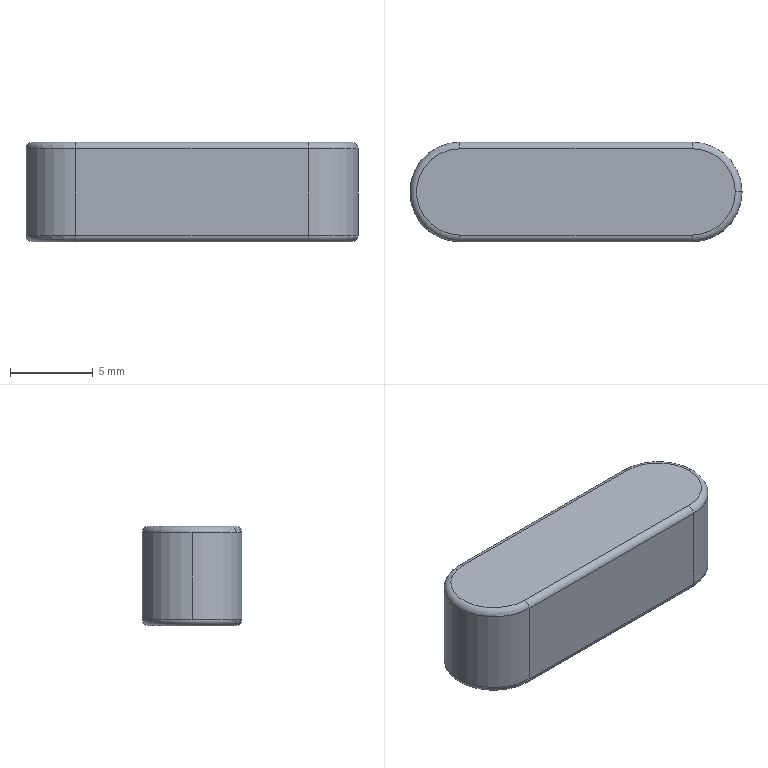Part | SolidWorks | features BaseBody 1 | 1 solid | 17 faces | box 20 x 6 x 6 mm | volume 670.467 mm3 | cylinder 7 | torus 6 | plane 4 | commonest cylinder face diameters 0.8 x4 6 x3
STEP:
#1=CARTESIAN_POINT('',(9.6,0.,0.));
#2=VERTEX_POINT('',#1);
#3=CARTESIAN_POINT('',(10.,0.,0.4));
#4=VERTEX_POINT('',#3);
#5=CARTESIAN_POINT('',(9.6,0.,0.4));
#6=DIRECTION('',(0.,-1.,0.));
#7=DIRECTION('',(0.,0.,-1.));
#8=AXIS2_PLACEMENT_3D('',#5,#6,#7);
#9=CIRCLE('',#8,0.4);
#10=EDGE_CURVE('',#2,#4,#9,.T.);
#11=ORIENTED_EDGE('',*,*,#10,.F.);
#12=CARTESIAN_POINT('',(7.,2.6,0.));
#13=VERTEX_POINT('',#12);
#14=CARTESIAN_POINT('',(7.,0.,0.));
#15=DIRECTION('',(0.,0.,-1.));
#16=DIRECTION('',(1.,0.,0.));
#17=AXIS2_PLACEMENT_3D('',#14,#15,#16);
#18=CIRCLE('',#17,2.6);
#19=EDGE_CURVE('',#13,#2,#18,.T.);
#20=ORIENTED_EDGE('',*,*,#19,.F.);
#21=CARTESIAN_POINT('',(7.,3.,0.4));
#22=VERTEX_POINT('',#21);
#23=CARTESIAN_POINT('',(7.,2.6,0.4));
#24=DIRECTION('',(1.,0.,0.));
#25=DIRECTION('',(0.,0.,-1.));
#26=AXIS2_PLACEMENT_3D('',#23,#24,#25);
#27=CIRCLE('',#26,0.4);
#28=EDGE_CURVE('',#13,#22,#27,.T.);
#29=ORIENTED_EDGE('',*,*,#28,.T.);
#30=CARTESIAN_POINT('',(7.,0.,0.4));
#31=DIRECTION('',(0.,0.,1.));
#32=DIRECTION('',(1.,0.,0.));
#33=AXIS2_PLACEMENT_3D('',#30,#31,#32);
#34=CIRCLE('',#33,3.);
#35=EDGE_CURVE('',#4,#22,#34,.T.);
#36=ORIENTED_EDGE('',*,*,#35,.F.);
#37=EDGE_LOOP('',(#11,#20,#29,#36));
#38=FACE_OUTER_BOUND('',#37,.T.);
#39=CARTESIAN_POINT('',(7.,0.,0.4));
#40=DIRECTION('',(0.,0.,1.));
#41=DIRECTION('',(1.,0.,0.));
#42=AXIS2_PLACEMENT_3D('',#39,#40,#41);
#43=TOROIDAL_SURFACE('',#42,2.6,0.4);
#44=ADVANCED_FACE('',(#38),#43,.T.);
#45=CARTESIAN_POINT('',(-7.,2.6,0.));
#46=VERTEX_POINT('',#45);
#47=CARTESIAN_POINT('',(-7.,3.,0.4));
#48=VERTEX_POINT('',#47);
#49=CARTESIAN_POINT('',(-7.,2.6,0.4));
#50=DIRECTION('',(1.,0.,0.));
#51=DIRECTION('',(0.,0.,-1.));
#52=AXIS2_PLACEMENT_3D('',#49,#50,#51);
#53=CIRCLE('',#52,0.4);
#54=EDGE_CURVE('',#46,#48,#53,.T.);
#55=ORIENTED_EDGE('',*,*,#54,.T.);
#56=CARTESIAN_POINT('',(-7.,3.,0.4));
#57=DIRECTION('',(-1.,0.,0.));
#58=VECTOR('',#57,1000.);
#59=LINE('',#56,#58);
#60=EDGE_CURVE('',#22,#48,#59,.T.);
#61=ORIENTED_EDGE('',*,*,#60,.F.);
#62=ORIENTED_EDGE('',*,*,#28,.F.);
#63=CARTESIAN_POINT('',(-7.,2.6,0.));
#64=DIRECTION('',(1.,0.,0.));
#65=VECTOR('',#64,1000.);
#66=LINE('',#63,#65);
#67=EDGE_CURVE('',#46,#13,#66,.T.);
#68=ORIENTED_EDGE('',*,*,#67,.F.);
#69=EDGE_LOOP('',(#55,#61,#62,#68));
#70=FACE_OUTER_BOUND('',#69,.T.);
#71=CARTESIAN_POINT('',(-7.,2.6,0.4));
#72=DIRECTION('',(-1.,0.,0.));
#73=DIRECTION('',(0.,-1.,0.));
#74=AXIS2_PLACEMENT_3D('',#71,#72,#73);
#75=CYLINDRICAL_SURFACE('',#74,0.4);
#76=ADVANCED_FACE('',(#70),#75,.T.);
#77=CARTESIAN_POINT('',(-7.,-3.,0.4));
#78=VERTEX_POINT('',#77);
#79=CARTESIAN_POINT('',(-7.,-2.6,0.));
#80=VERTEX_POINT('',#79);
#81=CARTESIAN_POINT('',(-7.,-2.6,0.4));
#82=DIRECTION('',(1.,0.,0.));
#83=DIRECTION('',(0.,0.,-1.));
#84=AXIS2_PLACEMENT_3D('',#81,#82,#83);
#85=CIRCLE('',#84,0.4);
#86=EDGE_CURVE('',#78,#80,#85,.T.);
#87=ORIENTED_EDGE('',*,*,#86,.T.);
#88=CARTESIAN_POINT('',(7.,-2.6,0.));
#89=VERTEX_POINT('',#88);
#90=CARTESIAN_POINT('',(-7.,-2.6,0.));
#91=DIRECTION('',(-1.,0.,0.));
#92=VECTOR('',#91,1000.);
#93=LINE('',#90,#92);
#94=EDGE_CURVE('',#89,#80,#93,.T.);
#95=ORIENTED_EDGE('',*,*,#94,.F.);
#96=CARTESIAN_POINT('',(7.,-3.,0.4));
#97=VERTEX_POINT('',#96);
#98=CARTESIAN_POINT('',(7.,-2.6,0.4));
#99=DIRECTION('',(1.,0.,0.));
#100=DIRECTION('',(0.,0.,-1.));
#101=AXIS2_PLACEMENT_3D('',#98,#99,#100);
#102=CIRCLE('',#101,0.4);
#103=EDGE_CURVE('',#97,#89,#102,.T.);
#104=ORIENTED_EDGE('',*,*,#103,.F.);
#105=CARTESIAN_POINT('',(-7.,-3.,0.4));
#106=DIRECTION('',(1.,0.,0.));
#107=VECTOR('',#106,1000.);
#108=LINE('',#105,#107);
#109=EDGE_CURVE('',#78,#97,#108,.T.);
#110=ORIENTED_EDGE('',*,*,#109,.F.);
#111=EDGE_LOOP('',(#87,#95,#104,#110));
#112=FACE_OUTER_BOUND('',#111,.T.);
#113=CARTESIAN_POINT('',(-7.,-2.6,0.4));
#114=DIRECTION('',(1.,0.,0.));
#115=DIRECTION('',(0.,1.,0.));
#116=AXIS2_PLACEMENT_3D('',#113,#114,#115);
#117=CYLINDRICAL_SURFACE('',#116,0.4);
#118=ADVANCED_FACE('',(#112),#117,.T.);
#119=ORIENTED_EDGE('',*,*,#54,.F.);
#120=CARTESIAN_POINT('',(-7.,0.,0.));
#121=DIRECTION('',(0.,0.,-1.));
#122=DIRECTION('',(1.,0.,0.));
#123=AXIS2_PLACEMENT_3D('',#120,#121,#122);
#124=CIRCLE('',#123,2.6);
#125=EDGE_CURVE('',#80,#46,#124,.T.);
#126=ORIENTED_EDGE('',*,*,#125,.F.);
#127=ORIENTED_EDGE('',*,*,#86,.F.);
#128=CARTESIAN_POINT('',(-10.,0.,0.4));
#129=VERTEX_POINT('',#128);
#130=CARTESIAN_POINT('',(-7.,0.,0.4));
#131=DIRECTION('',(0.,0.,1.));
#132=DIRECTION('',(1.,0.,0.));
#133=AXIS2_PLACEMENT_3D('',#130,#131,#132);
#134=CIRCLE('',#133,3.);
#135=EDGE_CURVE('',#129,#78,#134,.T.);
#136=ORIENTED_EDGE('',*,*,#135,.F.);
#137=CARTESIAN_POINT('',(-7.,0.,0.4));
#138=DIRECTION('',(0.,0.,1.));
#139=DIRECTION('',(1.,0.,0.));
#140=AXIS2_PLACEMENT_3D('',#137,#138,#139);
#141=CIRCLE('',#140,3.);
#142=EDGE_CURVE('',#48,#129,#141,.T.);
#143=ORIENTED_EDGE('',*,*,#142,.F.);
#144=EDGE_LOOP('',(#119,#126,#127,#136,#143));
#145=FACE_OUTER_BOUND('',#144,.T.);
#146=CARTESIAN_POINT('',(-7.,0.,0.4));
#147=DIRECTION('',(0.,0.,1.));
#148=DIRECTION('',(1.,0.,0.));
#149=AXIS2_PLACEMENT_3D('',#146,#147,#148);
#150=TOROIDAL_SURFACE('',#149,2.6,0.4);
#151=ADVANCED_FACE('',(#145),#150,.T.);
#152=CARTESIAN_POINT('',(10.,0.,5.6));
#153=VERTEX_POINT('',#152);
#154=CARTESIAN_POINT('',(9.6,0.,6.));
#155=VERTEX_POINT('',#154);
#156=CARTESIAN_POINT('',(9.6,0.,5.6));
#157=DIRECTION('',(0.,-1.,0.));
#158=DIRECTION('',(0.,0.,-1.));
#159=AXIS2_PLACEMENT_3D('',#156,#157,#158);
#160=CIRCLE('',#159,0.4);
#161=EDGE_CURVE('',#153,#155,#160,.T.);
#162=ORIENTED_EDGE('',*,*,#161,.F.);
#163=CARTESIAN_POINT('',(7.,3.,5.6));
#164=VERTEX_POINT('',#163);
#165=CARTESIAN_POINT('',(7.,0.,5.6));
#166=DIRECTION('',(0.,0.,-1.));
#167=DIRECTION('',(1.,0.,0.));
#168=AXIS2_PLACEMENT_3D('',#165,#166,#167);
#169=CIRCLE('',#168,3.);
#170=EDGE_CURVE('',#164,#153,#169,.T.);
#171=ORIENTED_EDGE('',*,*,#170,.F.);
#172=CARTESIAN_POINT('',(7.,2.6,6.));
#173=VERTEX_POINT('',#172);
#174=CARTESIAN_POINT('',(7.,2.6,5.6));
#175=DIRECTION('',(1.,0.,0.));
#176=DIRECTION('',(0.,0.,-1.));
#177=AXIS2_PLACEMENT_3D('',#174,#175,#176);
#178=CIRCLE('',#177,0.4);
#179=EDGE_CURVE('',#164,#173,#178,.T.);
#180=ORIENTED_EDGE('',*,*,#179,.T.);
#181=CARTESIAN_POINT('',(7.,0.,6.));
#182=DIRECTION('',(0.,0.,1.));
#183=DIRECTION('',(1.,0.,0.));
#184=AXIS2_PLACEMENT_3D('',#181,#182,#183);
#185=CIRCLE('',#184,2.6);
#186=EDGE_CURVE('',#155,#173,#185,.T.);
#187=ORIENTED_EDGE('',*,*,#186,.F.);
#188=EDGE_LOOP('',(#162,#171,#180,#187));
#189=FACE_OUTER_BOUND('',#188,.T.);
#190=CARTESIAN_POINT('',(7.,0.,5.6));
#191=DIRECTION('',(0.,0.,1.));
#192=DIRECTION('',(1.,0.,0.));
#193=AXIS2_PLACEMENT_3D('',#190,#191,#192);
#194=TOROIDAL_SURFACE('',#193,2.6,0.4);
#195=ADVANCED_FACE('',(#189),#194,.T.);
#196=CARTESIAN_POINT('',(-7.,3.,5.6));
#197=VERTEX_POINT('',#196);
#198=CARTESIAN_POINT('',(-7.,2.6,6.));
#199=VERTEX_POINT('',#198);
#200=CARTESIAN_POINT('',(-7.,2.6,5.6));
#201=DIRECTION('',(1.,0.,0.));
#202=DIRECTION('',(0.,0.,-1.));
#203=AXIS2_PLACEMENT_3D('',#200,#201,#202);
#204=CIRCLE('',#203,0.4);
#205=EDGE_CURVE('',#197,#199,#204,.T.);
#206=ORIENTED_EDGE('',*,*,#205,.T.);
#207=CARTESIAN_POINT('',(-7.,2.6,6.));
#208=DIRECTION('',(-1.,0.,0.));
#209=VECTOR('',#208,1000.);
#210=LINE('',#207,#209);
#211=EDGE_CURVE('',#173,#199,#210,.T.);
#212=ORIENTED_EDGE('',*,*,#211,.F.);
#213=ORIENTED_EDGE('',*,*,#179,.F.);
#214=CARTESIAN_POINT('',(7.,3.,5.6));
#215=DIRECTION('',(1.,0.,0.));
#216=VECTOR('',#215,1000.);
#217=LINE('',#214,#216);
#218=EDGE_CURVE('',#197,#164,#217,.T.);
#219=ORIENTED_EDGE('',*,*,#218,.F.);
#220=EDGE_LOOP('',(#206,#212,#213,#219));
#221=FACE_OUTER_BOUND('',#220,.T.);
#222=CARTESIAN_POINT('',(-7.,2.6,5.6));
#223=DIRECTION('',(1.,0.,0.));
#224=DIRECTION('',(0.,1.,0.));
#225=AXIS2_PLACEMENT_3D('',#222,#223,#224);
#226=CYLINDRICAL_SURFACE('',#225,0.4);
#227=ADVANCED_FACE('',(#221),#226,.T.);
#228=CARTESIAN_POINT('',(-7.,-2.6,6.));
#229=VERTEX_POINT('',#228);
#230=CARTESIAN_POINT('',(-7.,-3.,5.6));
#231=VERTEX_POINT('',#230);
#232=CARTESIAN_POINT('',(-7.,-2.6,5.6));
#233=DIRECTION('',(1.,0.,0.));
#234=DIRECTION('',(0.,0.,-1.));
#235=AXIS2_PLACEMENT_3D('',#232,#233,#234);
#236=CIRCLE('',#235,0.4);
#237=EDGE_CURVE('',#229,#231,#236,.T.);
#238=ORIENTED_EDGE('',*,*,#237,.T.);
#239=CARTESIAN_POINT('',(7.,-3.,5.6));
#240=VERTEX_POINT('',#239);
#241=CARTESIAN_POINT('',(-7.,-3.,5.6));
#242=DIRECTION('',(-1.,0.,0.));
#243=VECTOR('',#242,1000.);
#244=LINE('',#241,#243);
#245=EDGE_CURVE('',#240,#231,#244,.T.);
#246=ORIENTED_EDGE('',*,*,#245,.F.);
#247=CARTESIAN_POINT('',(7.,-2.6,6.));
#248=VERTEX_POINT('',#247);
#249=CARTESIAN_POINT('',(7.,-2.6,5.6));
#250=DIRECTION('',(1.,0.,0.));
#251=DIRECTION('',(0.,0.,-1.));
#252=AXIS2_PLACEMENT_3D('',#249,#250,#251);
#253=CIRCLE('',#252,0.4);
#254=EDGE_CURVE('',#248,#240,#253,.T.);
#255=ORIENTED_EDGE('',*,*,#254,.F.);
#256=CARTESIAN_POINT('',(7.,-2.6,6.));
#257=DIRECTION('',(1.,0.,0.));
#258=VECTOR('',#257,1000.);
#259=LINE('',#256,#258);
#260=EDGE_CURVE('',#229,#248,#259,.T.);
#261=ORIENTED_EDGE('',*,*,#260,.F.);
#262=EDGE_LOOP('',(#238,#246,#255,#261));
#263=FACE_OUTER_BOUND('',#262,.T.);
#264=CARTESIAN_POINT('',(-7.,-2.6,5.6));
#265=DIRECTION('',(-1.,0.,0.));
#266=DIRECTION('',(0.,-1.,0.));
#267=AXIS2_PLACEMENT_3D('',#264,#265,#266);
#268=CYLINDRICAL_SURFACE('',#267,0.4);
#269=ADVANCED_FACE('',(#263),#268,.T.);
#270=ORIENTED_EDGE('',*,*,#205,.F.);
#271=CARTESIAN_POINT('',(-10.,0.,5.6));
#272=VERTEX_POINT('',#271);
#273=CARTESIAN_POINT('',(-7.,0.,5.6));
#274=DIRECTION('',(0.,0.,-1.));
#275=DIRECTION('',(1.,0.,0.));
#276=AXIS2_PLACEMENT_3D('',#273,#274,#275);
#277=CIRCLE('',#276,3.);
#278=EDGE_CURVE('',#272,#197,#277,.T.);
#279=ORIENTED_EDGE('',*,*,#278,.F.);
#280=CARTESIAN_POINT('',(-7.,0.,5.6));
#281=DIRECTION('',(0.,0.,-1.));
#282=DIRECTION('',(1.,0.,0.));
#283=AXIS2_PLACEMENT_3D('',#280,#281,#282);
#284=CIRCLE('',#283,3.);
#285=EDGE_CURVE('',#231,#272,#284,.T.);
#286=ORIENTED_EDGE('',*,*,#285,.F.);
#287=ORIENTED_EDGE('',*,*,#237,.F.);
#288=CARTESIAN_POINT('',(-7.,0.,6.));
#289=DIRECTION('',(0.,0.,1.));
#290=DIRECTION('',(1.,0.,0.));
#291=AXIS2_PLACEMENT_3D('',#288,#289,#290);
#292=CIRCLE('',#291,2.6);
#293=EDGE_CURVE('',#199,#229,#292,.T.);
#294=ORIENTED_EDGE('',*,*,#293,.F.);
#295=EDGE_LOOP('',(#270,#279,#286,#287,#294));
#296=FACE_OUTER_BOUND('',#295,.T.);
#297=CARTESIAN_POINT('',(-7.,0.,5.6));
#298=DIRECTION('',(0.,0.,1.));
#299=DIRECTION('',(1.,0.,0.));
#300=AXIS2_PLACEMENT_3D('',#297,#298,#299);
#301=TOROIDAL_SURFACE('',#300,2.6,0.4);
#302=ADVANCED_FACE('',(#296),#301,.T.);
#303=ORIENTED_EDGE('',*,*,#67,.T.);
#304=ORIENTED_EDGE('',*,*,#19,.T.);
#305=CARTESIAN_POINT('',(7.,0.,0.));
#306=DIRECTION('',(0.,0.,-1.));
#307=DIRECTION('',(1.,0.,0.));
#308=AXIS2_PLACEMENT_3D('',#305,#306,#307);
#309=CIRCLE('',#308,2.6);
#310=EDGE_CURVE('',#2,#89,#309,.T.);
#311=ORIENTED_EDGE('',*,*,#310,.T.);
#312=ORIENTED_EDGE('',*,*,#94,.T.);
#313=ORIENTED_EDGE('',*,*,#125,.T.);
#314=EDGE_LOOP('',(#303,#304,#311,#312,#313));
#315=FACE_OUTER_BOUND('',#314,.T.);
#316=CARTESIAN_POINT('',(-7.,0.,0.));
#317=DIRECTION('',(0.,0.,1.));
#318=DIRECTION('',(0.,-1.,0.));
#319=AXIS2_PLACEMENT_3D('',#316,#317,#318);
#320=PLANE('',#319);
#321=ADVANCED_FACE('',(#315),#320,.F.);
#322=ORIENTED_EDGE('',*,*,#260,.T.);
#323=CARTESIAN_POINT('',(7.,0.,6.));
#324=DIRECTION('',(0.,0.,1.));
#325=DIRECTION('',(1.,0.,0.));
#326=AXIS2_PLACEMENT_3D('',#323,#324,#325);
#327=CIRCLE('',#326,2.6);
#328=EDGE_CURVE('',#248,#155,#327,.T.);
#329=ORIENTED_EDGE('',*,*,#328,.T.);
#330=ORIENTED_EDGE('',*,*,#186,.T.);
#331=ORIENTED_EDGE('',*,*,#211,.T.);
#332=ORIENTED_EDGE('',*,*,#293,.T.);
#333=EDGE_LOOP('',(#322,#329,#330,#331,#332));
#334=FACE_OUTER_BOUND('',#333,.T.);
#335=CARTESIAN_POINT('',(-7.,0.,6.));
#336=DIRECTION('',(0.,0.,1.));
#337=DIRECTION('',(0.,-1.,0.));
#338=AXIS2_PLACEMENT_3D('',#335,#336,#337);
#339=PLANE('',#338);
#340=ADVANCED_FACE('',(#334),#339,.T.);
#341=CARTESIAN_POINT('',(-7.,3.,6.));
#342=DIRECTION('',(0.,0.,-1.));
#343=VECTOR('',#342,1000.);
#344=LINE('',#341,#343);
#345=EDGE_CURVE('',#197,#48,#344,.T.);
#346=ORIENTED_EDGE('',*,*,#345,.F.);
#347=ORIENTED_EDGE('',*,*,#218,.T.);
#348=CARTESIAN_POINT('',(7.,3.,6.));
#349=DIRECTION('',(0.,0.,-1.));
#350=VECTOR('',#349,1000.);
#351=LINE('',#348,#350);
#352=EDGE_CURVE('',#164,#22,#351,.T.);
#353=ORIENTED_EDGE('',*,*,#352,.T.);
#354=ORIENTED_EDGE('',*,*,#60,.T.);
#355=EDGE_LOOP('',(#346,#347,#353,#354));
#356=FACE_OUTER_BOUND('',#355,.T.);
#357=CARTESIAN_POINT('',(-7.,3.,6.));
#358=DIRECTION('',(0.,-1.,0.));
#359=DIRECTION('',(0.,0.,-1.));
#360=AXIS2_PLACEMENT_3D('',#357,#358,#359);
#361=PLANE('',#360);
#362=ADVANCED_FACE('',(#356),#361,.F.);
#363=ORIENTED_EDGE('',*,*,#352,.F.);
#364=ORIENTED_EDGE('',*,*,#170,.T.);
#365=CARTESIAN_POINT('',(7.,0.,5.6));
#366=DIRECTION('',(0.,0.,-1.));
#367=DIRECTION('',(1.,0.,0.));
#368=AXIS2_PLACEMENT_3D('',#365,#366,#367);
#369=CIRCLE('',#368,3.);
#370=EDGE_CURVE('',#153,#240,#369,.T.);
#371=ORIENTED_EDGE('',*,*,#370,.T.);
#372=CARTESIAN_POINT('',(7.,-3.,6.));
#373=DIRECTION('',(0.,0.,-1.));
#374=VECTOR('',#373,1000.);
#375=LINE('',#372,#374);
#376=EDGE_CURVE('',#240,#97,#375,.T.);
#377=ORIENTED_EDGE('',*,*,#376,.T.);
#378=CARTESIAN_POINT('',(7.,0.,0.4));
#379=DIRECTION('',(0.,0.,1.));
#380=DIRECTION('',(1.,0.,0.));
#381=AXIS2_PLACEMENT_3D('',#378,#379,#380);
#382=CIRCLE('',#381,3.);
#383=EDGE_CURVE('',#97,#4,#382,.T.);
#384=ORIENTED_EDGE('',*,*,#383,.T.);
#385=ORIENTED_EDGE('',*,*,#35,.T.);
#386=EDGE_LOOP('',(#363,#364,#371,#377,#384,#385));
#387=FACE_OUTER_BOUND('',#386,.T.);
#388=CARTESIAN_POINT('',(7.,0.,6.));
#389=DIRECTION('',(0.,0.,-1.));
#390=DIRECTION('',(-1.,0.,0.));
#391=AXIS2_PLACEMENT_3D('',#388,#389,#390);
#392=CYLINDRICAL_SURFACE('',#391,3.);
#393=ADVANCED_FACE('',(#387),#392,.T.);
#394=ORIENTED_EDGE('',*,*,#376,.F.);
#395=ORIENTED_EDGE('',*,*,#245,.T.);
#396=CARTESIAN_POINT('',(-7.,-3.,6.));
#397=DIRECTION('',(0.,0.,-1.));
#398=VECTOR('',#397,1000.);
#399=LINE('',#396,#398);
#400=EDGE_CURVE('',#231,#78,#399,.T.);
#401=ORIENTED_EDGE('',*,*,#400,.T.);
#402=ORIENTED_EDGE('',*,*,#109,.T.);
#403=EDGE_LOOP('',(#394,#395,#401,#402));
#404=FACE_OUTER_BOUND('',#403,.T.);
#405=CARTESIAN_POINT('',(-7.,-3.,6.));
#406=DIRECTION('',(0.,1.,0.));
#407=DIRECTION('',(1.,0.,0.));
#408=AXIS2_PLACEMENT_3D('',#405,#406,#407);
#409=PLANE('',#408);
#410=ADVANCED_FACE('',(#404),#409,.F.);
#411=CARTESIAN_POINT('',(-10.,0.,6.));
#412=DIRECTION('',(0.,0.,-1.));
#413=VECTOR('',#412,1000.);
#414=LINE('',#411,#413);
#415=EDGE_CURVE('',#272,#129,#414,.T.);
#416=ORIENTED_EDGE('',*,*,#415,.F.);
#417=ORIENTED_EDGE('',*,*,#278,.T.);
#418=ORIENTED_EDGE('',*,*,#345,.T.);
#419=ORIENTED_EDGE('',*,*,#142,.T.);
#420=EDGE_LOOP('',(#416,#417,#418,#419));
#421=FACE_OUTER_BOUND('',#420,.T.);
#422=CARTESIAN_POINT('',(-7.,0.,6.));
#423=DIRECTION('',(0.,0.,-1.));
#424=DIRECTION('',(-1.,0.,0.));
#425=AXIS2_PLACEMENT_3D('',#422,#423,#424);
#426=CYLINDRICAL_SURFACE('',#425,3.);
#427=ADVANCED_FACE('',(#421),#426,.T.);
#428=ORIENTED_EDGE('',*,*,#285,.T.);
#429=ORIENTED_EDGE('',*,*,#415,.T.);
#430=ORIENTED_EDGE('',*,*,#135,.T.);
#431=ORIENTED_EDGE('',*,*,#400,.F.);
#432=EDGE_LOOP('',(#428,#429,#430,#431));
#433=FACE_OUTER_BOUND('',#432,.T.);
#434=CARTESIAN_POINT('',(-7.,0.,6.));
#435=DIRECTION('',(0.,0.,-1.));
#436=DIRECTION('',(-1.,0.,0.));
#437=AXIS2_PLACEMENT_3D('',#434,#435,#436);
#438=CYLINDRICAL_SURFACE('',#437,3.);
#439=ADVANCED_FACE('',(#433),#438,.T.);
#440=ORIENTED_EDGE('',*,*,#370,.F.);
#441=ORIENTED_EDGE('',*,*,#161,.T.);
#442=ORIENTED_EDGE('',*,*,#328,.F.);
#443=ORIENTED_EDGE('',*,*,#254,.T.);
#444=EDGE_LOOP('',(#440,#441,#442,#443));
#445=FACE_OUTER_BOUND('',#444,.T.);
#446=CARTESIAN_POINT('',(7.,0.,5.6));
#447=DIRECTION('',(0.,0.,1.));
#448=DIRECTION('',(1.,0.,0.));
#449=AXIS2_PLACEMENT_3D('',#446,#447,#448);
#450=TOROIDAL_SURFACE('',#449,2.6,0.4);
#451=ADVANCED_FACE('',(#445),#450,.T.);
#452=ORIENTED_EDGE('',*,*,#310,.F.);
#453=ORIENTED_EDGE('',*,*,#10,.T.);
#454=ORIENTED_EDGE('',*,*,#383,.F.);
#455=ORIENTED_EDGE('',*,*,#103,.T.);
#456=EDGE_LOOP('',(#452,#453,#454,#455));
#457=FACE_OUTER_BOUND('',#456,.T.);
#458=CARTESIAN_POINT('',(7.,0.,0.4));
#459=DIRECTION('',(0.,0.,1.));
#460=DIRECTION('',(1.,0.,0.));
#461=AXIS2_PLACEMENT_3D('',#458,#459,#460);
#462=TOROIDAL_SURFACE('',#461,2.6,0.4);
#463=ADVANCED_FACE('',(#457),#462,.T.);
#464=CLOSED_SHELL('',(#44,#76,#118,#151,#195,#227,#269,#302,#321,#340,#362,#393,#410,#427,#439,#451,#463));
#465=MANIFOLD_SOLID_BREP('',#464);
#466=CARTESIAN_POINT('',(0.,0.,0.));
#467=DIRECTION('',(0.,0.,1.));
#468=DIRECTION('',(1.,0.,0.));
#469=AXIS2_PLACEMENT_3D('',#466,#467,#468);
#470=(LENGTH_UNIT()NAMED_UNIT(*)SI_UNIT(.MILLI.,.METRE.));
#471=UNCERTAINTY_MEASURE_WITH_UNIT(LENGTH_MEASURE(0.00001),#470,'','');
#472=(NAMED_UNIT(*)PLANE_ANGLE_UNIT()SI_UNIT($,.RADIAN.));
#473=(NAMED_UNIT(*)SI_UNIT($,.STERADIAN.)SOLID_ANGLE_UNIT());
#474=(GEOMETRIC_REPRESENTATION_CONTEXT(3)GLOBAL_UNCERTAINTY_ASSIGNED_CONTEXT((#471))GLOBAL_UNIT_ASSIGNED_CONTEXT((#470,#472,#473))REPRESENTATION_CONTEXT('',''));
#475=ADVANCED_BREP_SHAPE_REPRESENTATION('',(#465,#469),#474);